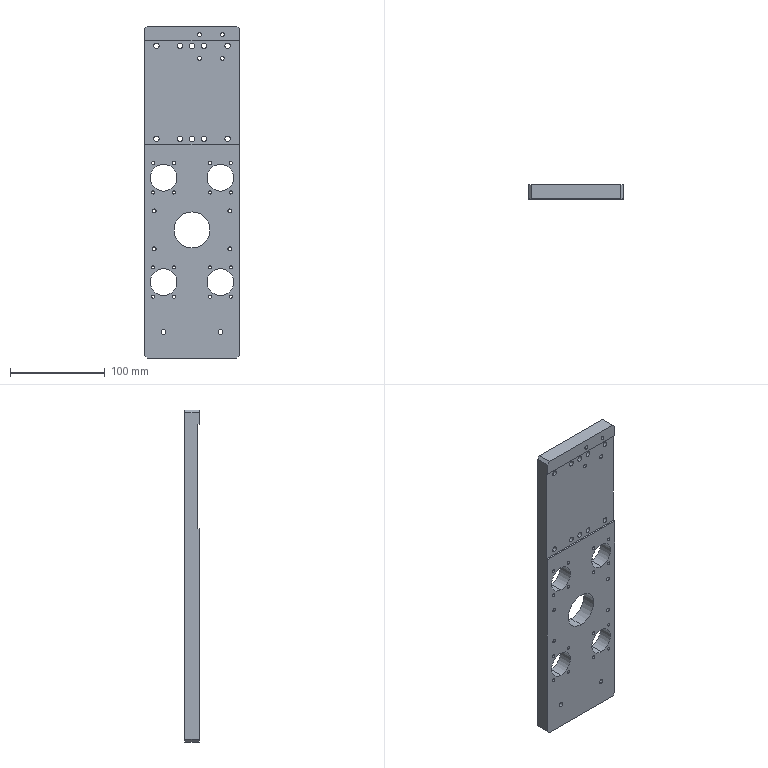Part | SolidWorks | features HoleWzd 6, ICE 3, Chamfer 1, Extrusion 1 | 1 solid | 120 faces | box 100 x 15 x 350 mm | volume 438251 mm3 | cylinder 98 | plane 22 | commonest cylinder face diameters 3.3 x32 4.2 x16 5.5 x16 10 x16 28.2 x8 5 x4